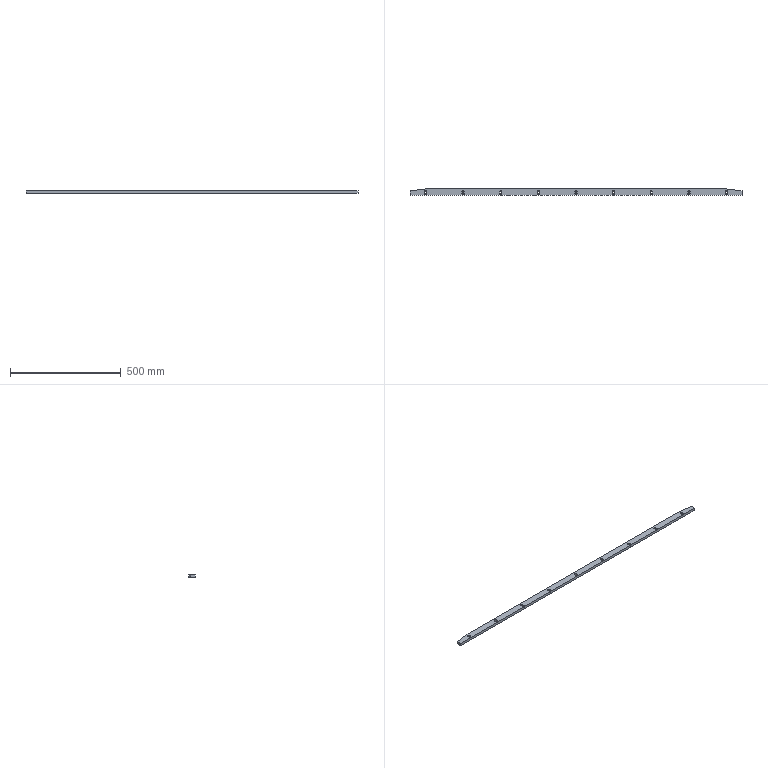Part | STEP file | Outer nylon backrest plate 2 | 1 solid | 89 faces | box 1500 x 30 x 12 mm | volume 516633 mm3 | plane 53 | cylinder 36 | commonest cylinder face diameters 7 x18 11 x18